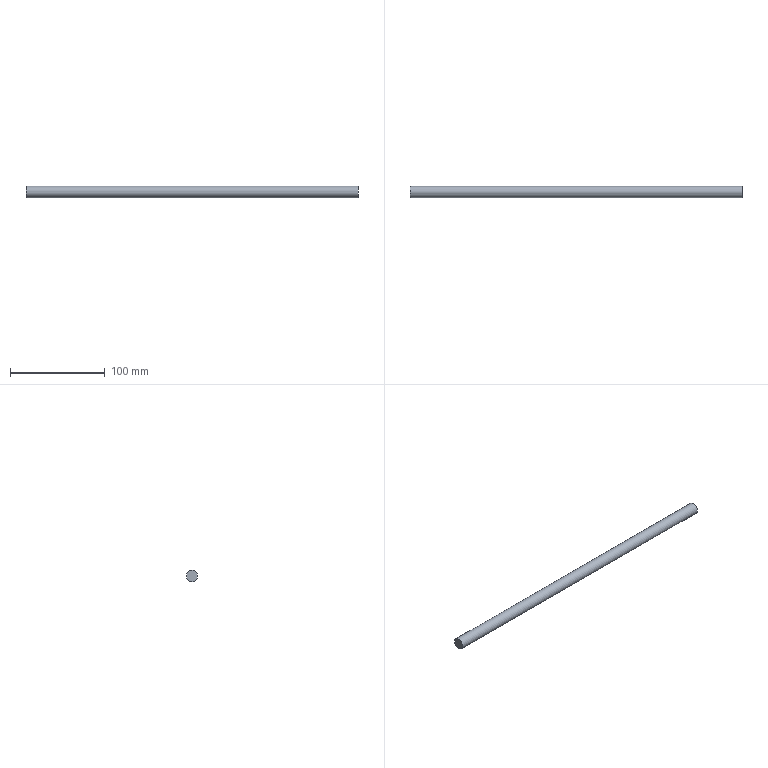Part | STEP file | 冲床-300配套压波_id474_x_t | 1 solid | 3 faces | box 350 x 12 x 12 mm | volume 39584 mm3 | plane 2 | cylinder 1 | commonest cylinder face diameters 12 x1
STEP:
#1=CARTESIAN_POINT('',(1153.,-102.,-108.));
#2=VERTEX_POINT('',#1);
#3=CARTESIAN_POINT('',(1153.,-102.,-114.));
#4=DIRECTION('',(1.,0.,0.));
#5=DIRECTION('',(0.,0.,1.));
#6=AXIS2_PLACEMENT_3D('',#3,#4,#5);
#7=CIRCLE('',#6,6.);
#8=EDGE_CURVE('',#2,#2,#7,.T.);
#9=ORIENTED_EDGE('',*,*,#8,.F.);
#10=EDGE_LOOP('',(#9));
#11=FACE_BOUND('',#10,.T.);
#12=CARTESIAN_POINT('',(803.,-102.,-108.));
#13=VERTEX_POINT('',#12);
#14=CARTESIAN_POINT('',(803.,-102.,-114.));
#15=DIRECTION('',(1.,0.,0.));
#16=DIRECTION('',(0.,0.,1.));
#17=AXIS2_PLACEMENT_3D('',#14,#15,#16);
#18=CIRCLE('',#17,6.);
#19=EDGE_CURVE('',#13,#13,#18,.T.);
#20=ORIENTED_EDGE('',*,*,#19,.T.);
#21=EDGE_LOOP('',(#20));
#22=FACE_BOUND('',#21,.T.);
#23=CARTESIAN_POINT('',(1172.,-102.,-114.));
#24=DIRECTION('',(-1.,0.,0.));
#25=DIRECTION('',(0.,0.,-1.));
#26=AXIS2_PLACEMENT_3D('',#23,#24,#25);
#27=CYLINDRICAL_SURFACE('',#26,6.);
#28=ADVANCED_FACE('',(#11,#22),#27,.T.);
#29=ORIENTED_EDGE('',*,*,#8,.T.);
#30=EDGE_LOOP('',(#29));
#31=FACE_OUTER_BOUND('',#30,.T.);
#32=CARTESIAN_POINT('',(1153.,-102.,-114.));
#33=DIRECTION('',(1.,0.,0.));
#34=DIRECTION('',(0.,0.,1.));
#35=AXIS2_PLACEMENT_3D('',#32,#33,#34);
#36=PLANE('',#35);
#37=ADVANCED_FACE('',(#31),#36,.T.);
#38=ORIENTED_EDGE('',*,*,#19,.F.);
#39=EDGE_LOOP('',(#38));
#40=FACE_OUTER_BOUND('',#39,.T.);
#41=CARTESIAN_POINT('',(803.,-102.,-114.));
#42=DIRECTION('',(1.,0.,0.));
#43=DIRECTION('',(0.,0.,1.));
#44=AXIS2_PLACEMENT_3D('',#41,#42,#43);
#45=PLANE('',#44);
#46=ADVANCED_FACE('',(#40),#45,.F.);
#47=CLOSED_SHELL('',(#28,#37,#46));
#48=MANIFOLD_SOLID_BREP('',#47);
#49=(LENGTH_UNIT()NAMED_UNIT(*)SI_UNIT(.MILLI.,.METRE.));
#50=UNCERTAINTY_MEASURE_WITH_UNIT(LENGTH_MEASURE(0.00002),#49,'','');
#51=(NAMED_UNIT(*)PLANE_ANGLE_UNIT()SI_UNIT($,.RADIAN.));
#52=PLANE_ANGLE_MEASURE_WITH_UNIT(PLANE_ANGLE_MEASURE(0.01745),#51);
#53=DIMENSIONAL_EXPONENTS(0.,0.,0.,0.,0.,0.,0.);
#54=(CONVERSION_BASED_UNIT('DEGREE',#52)NAMED_UNIT(#53)PLANE_ANGLE_UNIT());
#55=(NAMED_UNIT(*)SI_UNIT($,.STERADIAN.)SOLID_ANGLE_UNIT());
#56=(GEOMETRIC_REPRESENTATION_CONTEXT(3)GLOBAL_UNCERTAINTY_ASSIGNED_CONTEXT((#50))GLOBAL_UNIT_ASSIGNED_CONTEXT((#49,#54,#55))REPRESENTATION_CONTEXT('',''));
#57=ADVANCED_BREP_SHAPE_REPRESENTATION('',(#48),#56);